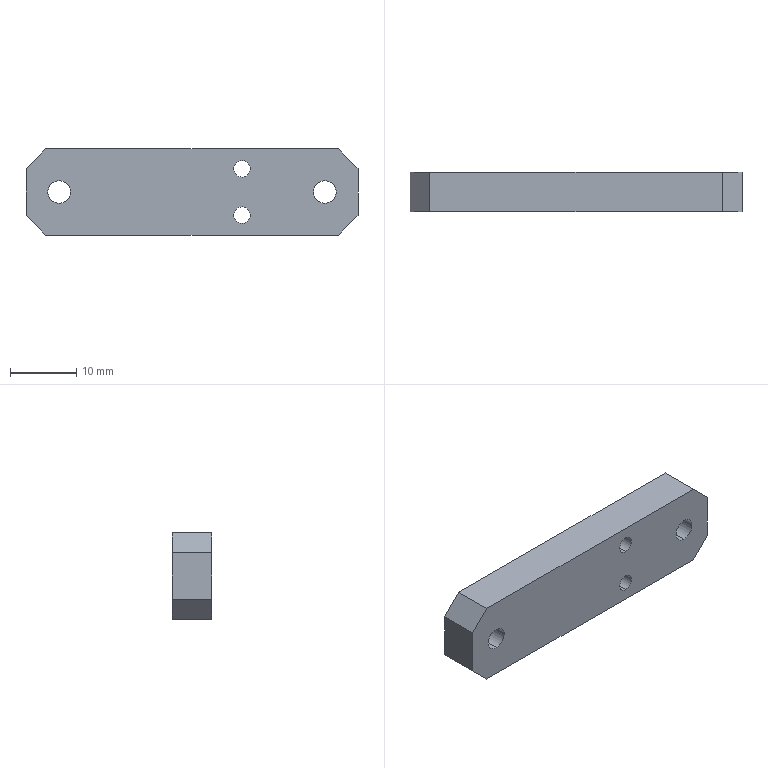Part | NX | features BREP 1 | 1 solid | 24 faces | box 50 x 6 x 13 mm | volume 3494 mm3 | cylinder 12 | plane 12 | commonest cylinder face diameters 2.5 x4 3.4 x4 6 x4
STEP:
#1=CARTESIAN_POINT('',(7.55,-3.,2.252));
#2=VERTEX_POINT('',#1);
#3=CARTESIAN_POINT('',(7.55,-3.,4.752));
#4=VERTEX_POINT('',#3);
#5=CARTESIAN_POINT('',(7.55,-3.,3.502));
#6=DIRECTION('',(0.,1.,0.));
#7=DIRECTION('',(0.,0.,1.));
#8=AXIS2_PLACEMENT_3D('',#5,#6,#7);
#9=CIRCLE('',#8,1.25);
#10=EDGE_CURVE('',#2,#4,#9,.T.);
#11=ORIENTED_EDGE('',*,*,#10,.F.);
#12=CARTESIAN_POINT('',(7.55,3.,2.252));
#13=VERTEX_POINT('',#12);
#14=CARTESIAN_POINT('',(7.55,3.,2.252));
#15=DIRECTION('',(0.,1.,0.));
#16=VECTOR('',#15,1000.);
#17=LINE('',#14,#16);
#18=EDGE_CURVE('',#2,#13,#17,.T.);
#19=ORIENTED_EDGE('',*,*,#18,.T.);
#20=CARTESIAN_POINT('',(7.55,3.,4.752));
#21=VERTEX_POINT('',#20);
#22=CARTESIAN_POINT('',(7.55,3.,3.502));
#23=DIRECTION('',(0.,1.,0.));
#24=DIRECTION('',(0.,0.,1.));
#25=AXIS2_PLACEMENT_3D('',#22,#23,#24);
#26=CIRCLE('',#25,1.25);
#27=EDGE_CURVE('',#13,#21,#26,.T.);
#28=ORIENTED_EDGE('',*,*,#27,.T.);
#29=CARTESIAN_POINT('',(7.55,3.,4.752));
#30=DIRECTION('',(0.,1.,0.));
#31=VECTOR('',#30,1000.);
#32=LINE('',#29,#31);
#33=EDGE_CURVE('',#4,#21,#32,.T.);
#34=ORIENTED_EDGE('',*,*,#33,.F.);
#35=EDGE_LOOP('',(#11,#19,#28,#34));
#36=FACE_BOUND('',#35,.T.);
#37=CARTESIAN_POINT('',(7.55,3.,3.502));
#38=DIRECTION('',(0.,1.,0.));
#39=DIRECTION('',(0.,0.,-1.));
#40=AXIS2_PLACEMENT_3D('',#37,#38,#39);
#41=CYLINDRICAL_SURFACE('',#40,1.25);
#42=ADVANCED_FACE('',(#36),#41,.F.);
#43=CARTESIAN_POINT('',(7.55,-3.,-4.752));
#44=VERTEX_POINT('',#43);
#45=CARTESIAN_POINT('',(7.55,-3.,-2.252));
#46=VERTEX_POINT('',#45);
#47=CARTESIAN_POINT('',(7.55,-3.,-3.502));
#48=DIRECTION('',(0.,1.,0.));
#49=DIRECTION('',(0.,0.,1.));
#50=AXIS2_PLACEMENT_3D('',#47,#48,#49);
#51=CIRCLE('',#50,1.25);
#52=EDGE_CURVE('',#44,#46,#51,.T.);
#53=ORIENTED_EDGE('',*,*,#52,.F.);
#54=CARTESIAN_POINT('',(7.55,3.,-4.752));
#55=VERTEX_POINT('',#54);
#56=CARTESIAN_POINT('',(7.55,3.,-4.752));
#57=DIRECTION('',(0.,1.,0.));
#58=VECTOR('',#57,1000.);
#59=LINE('',#56,#58);
#60=EDGE_CURVE('',#44,#55,#59,.T.);
#61=ORIENTED_EDGE('',*,*,#60,.T.);
#62=CARTESIAN_POINT('',(7.55,3.,-2.252));
#63=VERTEX_POINT('',#62);
#64=CARTESIAN_POINT('',(7.55,3.,-3.502));
#65=DIRECTION('',(0.,1.,0.));
#66=DIRECTION('',(0.,0.,1.));
#67=AXIS2_PLACEMENT_3D('',#64,#65,#66);
#68=CIRCLE('',#67,1.25);
#69=EDGE_CURVE('',#55,#63,#68,.T.);
#70=ORIENTED_EDGE('',*,*,#69,.T.);
#71=CARTESIAN_POINT('',(7.55,3.,-2.252));
#72=DIRECTION('',(0.,1.,0.));
#73=VECTOR('',#72,1000.);
#74=LINE('',#71,#73);
#75=EDGE_CURVE('',#46,#63,#74,.T.);
#76=ORIENTED_EDGE('',*,*,#75,.F.);
#77=EDGE_LOOP('',(#53,#61,#70,#76));
#78=FACE_BOUND('',#77,.T.);
#79=CARTESIAN_POINT('',(7.55,3.,-3.502));
#80=DIRECTION('',(0.,1.,0.));
#81=DIRECTION('',(0.,0.,-1.));
#82=AXIS2_PLACEMENT_3D('',#79,#80,#81);
#83=CYLINDRICAL_SURFACE('',#82,1.25);
#84=ADVANCED_FACE('',(#78),#83,.F.);
#85=CARTESIAN_POINT('',(-20.,-0.4,-3.));
#86=VERTEX_POINT('',#85);
#87=CARTESIAN_POINT('',(-20.,-0.4,3.));
#88=VERTEX_POINT('',#87);
#89=CARTESIAN_POINT('',(-20.,-0.4,0.));
#90=DIRECTION('',(0.,1.,0.));
#91=DIRECTION('',(0.,0.,1.));
#92=AXIS2_PLACEMENT_3D('',#89,#90,#91);
#93=CIRCLE('',#92,3.);
#94=EDGE_CURVE('',#86,#88,#93,.T.);
#95=ORIENTED_EDGE('',*,*,#94,.F.);
#96=CARTESIAN_POINT('',(-20.,3.,-3.));
#97=VERTEX_POINT('',#96);
#98=CARTESIAN_POINT('',(-20.,3.,-3.));
#99=DIRECTION('',(0.,1.,0.));
#100=VECTOR('',#99,1000.);
#101=LINE('',#98,#100);
#102=EDGE_CURVE('',#86,#97,#101,.T.);
#103=ORIENTED_EDGE('',*,*,#102,.T.);
#104=CARTESIAN_POINT('',(-20.,3.,3.));
#105=VERTEX_POINT('',#104);
#106=CARTESIAN_POINT('',(-20.,3.,0.));
#107=DIRECTION('',(0.,1.,0.));
#108=DIRECTION('',(0.,0.,1.));
#109=AXIS2_PLACEMENT_3D('',#106,#107,#108);
#110=CIRCLE('',#109,3.);
#111=EDGE_CURVE('',#97,#105,#110,.T.);
#112=ORIENTED_EDGE('',*,*,#111,.T.);
#113=CARTESIAN_POINT('',(-20.,3.,3.));
#114=DIRECTION('',(0.,1.,0.));
#115=VECTOR('',#114,1000.);
#116=LINE('',#113,#115);
#117=EDGE_CURVE('',#88,#105,#116,.T.);
#118=ORIENTED_EDGE('',*,*,#117,.F.);
#119=EDGE_LOOP('',(#95,#103,#112,#118));
#120=FACE_BOUND('',#119,.T.);
#121=CARTESIAN_POINT('',(-20.,3.,0.));
#122=DIRECTION('',(0.,1.,0.));
#123=DIRECTION('',(0.,0.,-1.));
#124=AXIS2_PLACEMENT_3D('',#121,#122,#123);
#125=CYLINDRICAL_SURFACE('',#124,3.);
#126=ADVANCED_FACE('',(#120),#125,.F.);
#127=CARTESIAN_POINT('',(-20.,-3.,-1.7));
#128=VERTEX_POINT('',#127);
#129=CARTESIAN_POINT('',(-20.,-3.,1.7));
#130=VERTEX_POINT('',#129);
#131=CARTESIAN_POINT('',(-20.,-3.,0.));
#132=DIRECTION('',(0.,1.,0.));
#133=DIRECTION('',(0.,0.,1.));
#134=AXIS2_PLACEMENT_3D('',#131,#132,#133);
#135=CIRCLE('',#134,1.7);
#136=EDGE_CURVE('',#128,#130,#135,.T.);
#137=ORIENTED_EDGE('',*,*,#136,.F.);
#138=CARTESIAN_POINT('',(-20.,-0.4,-1.7));
#139=VERTEX_POINT('',#138);
#140=CARTESIAN_POINT('',(-20.,3.,-1.7));
#141=DIRECTION('',(0.,1.,0.));
#142=VECTOR('',#141,1000.);
#143=LINE('',#140,#142);
#144=EDGE_CURVE('',#128,#139,#143,.T.);
#145=ORIENTED_EDGE('',*,*,#144,.T.);
#146=CARTESIAN_POINT('',(-20.,-0.4,1.7));
#147=VERTEX_POINT('',#146);
#148=CARTESIAN_POINT('',(-20.,-0.4,0.));
#149=DIRECTION('',(0.,1.,0.));
#150=DIRECTION('',(0.,0.,1.));
#151=AXIS2_PLACEMENT_3D('',#148,#149,#150);
#152=CIRCLE('',#151,1.7);
#153=EDGE_CURVE('',#139,#147,#152,.T.);
#154=ORIENTED_EDGE('',*,*,#153,.T.);
#155=CARTESIAN_POINT('',(-20.,3.,1.7));
#156=DIRECTION('',(0.,1.,0.));
#157=VECTOR('',#156,1000.);
#158=LINE('',#155,#157);
#159=EDGE_CURVE('',#130,#147,#158,.T.);
#160=ORIENTED_EDGE('',*,*,#159,.F.);
#161=EDGE_LOOP('',(#137,#145,#154,#160));
#162=FACE_BOUND('',#161,.T.);
#163=CARTESIAN_POINT('',(-20.,3.,0.));
#164=DIRECTION('',(0.,1.,0.));
#165=DIRECTION('',(0.,0.,-1.));
#166=AXIS2_PLACEMENT_3D('',#163,#164,#165);
#167=CYLINDRICAL_SURFACE('',#166,1.7);
#168=ADVANCED_FACE('',(#162),#167,.F.);
#169=CARTESIAN_POINT('',(20.,-0.4,-3.));
#170=VERTEX_POINT('',#169);
#171=CARTESIAN_POINT('',(20.,-0.4,3.));
#172=VERTEX_POINT('',#171);
#173=CARTESIAN_POINT('',(20.,-0.4,0.));
#174=DIRECTION('',(0.,1.,0.));
#175=DIRECTION('',(0.,0.,1.));
#176=AXIS2_PLACEMENT_3D('',#173,#174,#175);
#177=CIRCLE('',#176,3.);
#178=EDGE_CURVE('',#170,#172,#177,.T.);
#179=ORIENTED_EDGE('',*,*,#178,.F.);
#180=CARTESIAN_POINT('',(20.,3.,-3.));
#181=VERTEX_POINT('',#180);
#182=CARTESIAN_POINT('',(20.,3.,-3.));
#183=DIRECTION('',(0.,1.,0.));
#184=VECTOR('',#183,1000.);
#185=LINE('',#182,#184);
#186=EDGE_CURVE('',#170,#181,#185,.T.);
#187=ORIENTED_EDGE('',*,*,#186,.T.);
#188=CARTESIAN_POINT('',(20.,3.,3.));
#189=VERTEX_POINT('',#188);
#190=CARTESIAN_POINT('',(20.,3.,0.));
#191=DIRECTION('',(0.,1.,0.));
#192=DIRECTION('',(0.,0.,1.));
#193=AXIS2_PLACEMENT_3D('',#190,#191,#192);
#194=CIRCLE('',#193,3.);
#195=EDGE_CURVE('',#181,#189,#194,.T.);
#196=ORIENTED_EDGE('',*,*,#195,.T.);
#197=CARTESIAN_POINT('',(20.,3.,3.));
#198=DIRECTION('',(0.,1.,0.));
#199=VECTOR('',#198,1000.);
#200=LINE('',#197,#199);
#201=EDGE_CURVE('',#172,#189,#200,.T.);
#202=ORIENTED_EDGE('',*,*,#201,.F.);
#203=EDGE_LOOP('',(#179,#187,#196,#202));
#204=FACE_BOUND('',#203,.T.);
#205=CARTESIAN_POINT('',(20.,3.,0.));
#206=DIRECTION('',(0.,1.,0.));
#207=DIRECTION('',(0.,0.,-1.));
#208=AXIS2_PLACEMENT_3D('',#205,#206,#207);
#209=CYLINDRICAL_SURFACE('',#208,3.);
#210=ADVANCED_FACE('',(#204),#209,.F.);
#211=CARTESIAN_POINT('',(20.,-3.,-1.7));
#212=VERTEX_POINT('',#211);
#213=CARTESIAN_POINT('',(20.,-3.,1.7));
#214=VERTEX_POINT('',#213);
#215=CARTESIAN_POINT('',(20.,-3.,0.));
#216=DIRECTION('',(0.,1.,0.));
#217=DIRECTION('',(0.,0.,1.));
#218=AXIS2_PLACEMENT_3D('',#215,#216,#217);
#219=CIRCLE('',#218,1.7);
#220=EDGE_CURVE('',#212,#214,#219,.T.);
#221=ORIENTED_EDGE('',*,*,#220,.F.);
#222=CARTESIAN_POINT('',(20.,-0.4,-1.7));
#223=VERTEX_POINT('',#222);
#224=CARTESIAN_POINT('',(20.,3.,-1.7));
#225=DIRECTION('',(0.,1.,0.));
#226=VECTOR('',#225,1000.);
#227=LINE('',#224,#226);
#228=EDGE_CURVE('',#212,#223,#227,.T.);
#229=ORIENTED_EDGE('',*,*,#228,.T.);
#230=CARTESIAN_POINT('',(20.,-0.4,1.7));
#231=VERTEX_POINT('',#230);
#232=CARTESIAN_POINT('',(20.,-0.4,0.));
#233=DIRECTION('',(0.,1.,0.));
#234=DIRECTION('',(0.,0.,1.));
#235=AXIS2_PLACEMENT_3D('',#232,#233,#234);
#236=CIRCLE('',#235,1.7);
#237=EDGE_CURVE('',#223,#231,#236,.T.);
#238=ORIENTED_EDGE('',*,*,#237,.T.);
#239=CARTESIAN_POINT('',(20.,3.,1.7));
#240=DIRECTION('',(0.,1.,0.));
#241=VECTOR('',#240,1000.);
#242=LINE('',#239,#241);
#243=EDGE_CURVE('',#214,#231,#242,.T.);
#244=ORIENTED_EDGE('',*,*,#243,.F.);
#245=EDGE_LOOP('',(#221,#229,#238,#244));
#246=FACE_BOUND('',#245,.T.);
#247=CARTESIAN_POINT('',(20.,3.,0.));
#248=DIRECTION('',(0.,1.,0.));
#249=DIRECTION('',(0.,0.,-1.));
#250=AXIS2_PLACEMENT_3D('',#247,#248,#249);
#251=CYLINDRICAL_SURFACE('',#250,1.7);
#252=ADVANCED_FACE('',(#246),#251,.F.);
#253=CARTESIAN_POINT('',(25.,-3.,3.5));
#254=VERTEX_POINT('',#253);
#255=CARTESIAN_POINT('',(25.,-3.,-3.5));
#256=VERTEX_POINT('',#255);
#257=CARTESIAN_POINT('',(25.,-3.,-6.5));
#258=DIRECTION('',(0.,0.,-1.));
#259=VECTOR('',#258,1000.);
#260=LINE('',#257,#259);
#261=EDGE_CURVE('',#254,#256,#260,.T.);
#262=ORIENTED_EDGE('',*,*,#261,.T.);
#263=CARTESIAN_POINT('',(25.,3.,-3.5));
#264=VERTEX_POINT('',#263);
#265=CARTESIAN_POINT('',(25.,3.,-3.5));
#266=DIRECTION('',(0.,1.,0.));
#267=VECTOR('',#266,1000.);
#268=LINE('',#265,#267);
#269=EDGE_CURVE('',#256,#264,#268,.T.);
#270=ORIENTED_EDGE('',*,*,#269,.T.);
#271=CARTESIAN_POINT('',(25.,3.,3.5));
#272=VERTEX_POINT('',#271);
#273=CARTESIAN_POINT('',(25.,3.,-6.5));
#274=DIRECTION('',(0.,0.,-1.));
#275=VECTOR('',#274,1000.);
#276=LINE('',#273,#275);
#277=EDGE_CURVE('',#272,#264,#276,.T.);
#278=ORIENTED_EDGE('',*,*,#277,.F.);
#279=CARTESIAN_POINT('',(25.,3.,3.5));
#280=DIRECTION('',(0.,-1.,0.));
#281=VECTOR('',#280,1000.);
#282=LINE('',#279,#281);
#283=EDGE_CURVE('',#272,#254,#282,.T.);
#284=ORIENTED_EDGE('',*,*,#283,.T.);
#285=EDGE_LOOP('',(#262,#270,#278,#284));
#286=FACE_BOUND('',#285,.T.);
#287=CARTESIAN_POINT('',(25.,3.,-6.5));
#288=DIRECTION('',(-1.,0.,0.));
#289=DIRECTION('',(0.,0.,-1.));
#290=AXIS2_PLACEMENT_3D('',#287,#288,#289);
#291=PLANE('',#290);
#292=ADVANCED_FACE('',(#286),#291,.F.);
#293=CARTESIAN_POINT('',(22.,-3.,-6.5));
#294=VERTEX_POINT('',#293);
#295=CARTESIAN_POINT('',(-22.,-3.,-6.5));
#296=VERTEX_POINT('',#295);
#297=CARTESIAN_POINT('',(-25.,-3.,-6.5));
#298=DIRECTION('',(-1.,0.,0.));
#299=VECTOR('',#298,1000.);
#300=LINE('',#297,#299);
#301=EDGE_CURVE('',#294,#296,#300,.T.);
#302=ORIENTED_EDGE('',*,*,#301,.T.);
#303=CARTESIAN_POINT('',(-22.,3.,-6.5));
#304=VERTEX_POINT('',#303);
#305=CARTESIAN_POINT('',(-22.,3.,-6.5));
#306=DIRECTION('',(0.,1.,0.));
#307=VECTOR('',#306,1000.);
#308=LINE('',#305,#307);
#309=EDGE_CURVE('',#296,#304,#308,.T.);
#310=ORIENTED_EDGE('',*,*,#309,.T.);
#311=CARTESIAN_POINT('',(22.,3.,-6.5));
#312=VERTEX_POINT('',#311);
#313=CARTESIAN_POINT('',(-25.,3.,-6.5));
#314=DIRECTION('',(-1.,0.,0.));
#315=VECTOR('',#314,1000.);
#316=LINE('',#313,#315);
#317=EDGE_CURVE('',#312,#304,#316,.T.);
#318=ORIENTED_EDGE('',*,*,#317,.F.);
#319=CARTESIAN_POINT('',(22.,3.,-6.5));
#320=DIRECTION('',(0.,-1.,0.));
#321=VECTOR('',#320,1000.);
#322=LINE('',#319,#321);
#323=EDGE_CURVE('',#312,#294,#322,.T.);
#324=ORIENTED_EDGE('',*,*,#323,.T.);
#325=EDGE_LOOP('',(#302,#310,#318,#324));
#326=FACE_BOUND('',#325,.T.);
#327=CARTESIAN_POINT('',(-25.,3.,-6.5));
#328=DIRECTION('',(0.,0.,1.));
#329=DIRECTION('',(-1.,0.,0.));
#330=AXIS2_PLACEMENT_3D('',#327,#328,#329);
#331=PLANE('',#330);
#332=ADVANCED_FACE('',(#326),#331,.F.);
#333=CARTESIAN_POINT('',(-25.,-3.,-3.5));
#334=VERTEX_POINT('',#333);
#335=CARTESIAN_POINT('',(-25.,-3.,3.5));
#336=VERTEX_POINT('',#335);
#337=CARTESIAN_POINT('',(-25.,-3.,-6.5));
#338=DIRECTION('',(0.,0.,1.));
#339=VECTOR('',#338,1000.);
#340=LINE('',#337,#339);
#341=EDGE_CURVE('',#334,#336,#340,.T.);
#342=ORIENTED_EDGE('',*,*,#341,.T.);
#343=CARTESIAN_POINT('',(-25.,3.,3.5));
#344=VERTEX_POINT('',#343);
#345=CARTESIAN_POINT('',(-25.,3.,3.5));
#346=DIRECTION('',(0.,1.,0.));
#347=VECTOR('',#346,1000.);
#348=LINE('',#345,#347);
#349=EDGE_CURVE('',#336,#344,#348,.T.);
#350=ORIENTED_EDGE('',*,*,#349,.T.);
#351=CARTESIAN_POINT('',(-25.,3.,-3.5));
#352=VERTEX_POINT('',#351);
#353=CARTESIAN_POINT('',(-25.,3.,-6.5));
#354=DIRECTION('',(0.,0.,1.));
#355=VECTOR('',#354,1000.);
#356=LINE('',#353,#355);
#357=EDGE_CURVE('',#352,#344,#356,.T.);
#358=ORIENTED_EDGE('',*,*,#357,.F.);
#359=CARTESIAN_POINT('',(-25.,3.,-3.5));
#360=DIRECTION('',(0.,-1.,0.));
#361=VECTOR('',#360,1000.);
#362=LINE('',#359,#361);
#363=EDGE_CURVE('',#352,#334,#362,.T.);
#364=ORIENTED_EDGE('',*,*,#363,.T.);
#365=EDGE_LOOP('',(#342,#350,#358,#364));
#366=FACE_BOUND('',#365,.T.);
#367=CARTESIAN_POINT('',(-25.,3.,-6.5));
#368=DIRECTION('',(1.,0.,0.));
#369=DIRECTION('',(0.,0.,1.));
#370=AXIS2_PLACEMENT_3D('',#367,#368,#369);
#371=PLANE('',#370);
#372=ADVANCED_FACE('',(#366),#371,.F.);
#373=CARTESIAN_POINT('',(-22.,3.,6.5));
#374=VERTEX_POINT('',#373);
#375=CARTESIAN_POINT('',(22.,3.,6.5));
#376=VERTEX_POINT('',#375);
#377=CARTESIAN_POINT('',(-25.,3.,6.5));
#378=DIRECTION('',(1.,0.,0.));
#379=VECTOR('',#378,1000.);
#380=LINE('',#377,#379);
#381=EDGE_CURVE('',#374,#376,#380,.T.);
#382=ORIENTED_EDGE('',*,*,#381,.F.);
#383=CARTESIAN_POINT('',(-22.,-3.,6.5));
#384=VERTEX_POINT('',#383);
#385=CARTESIAN_POINT('',(-22.,3.,6.5));
#386=DIRECTION('',(0.,-1.,0.));
#387=VECTOR('',#386,1000.);
#388=LINE('',#385,#387);
#389=EDGE_CURVE('',#374,#384,#388,.T.);
#390=ORIENTED_EDGE('',*,*,#389,.T.);
#391=CARTESIAN_POINT('',(22.,-3.,6.5));
#392=VERTEX_POINT('',#391);
#393=CARTESIAN_POINT('',(-25.,-3.,6.5));
#394=DIRECTION('',(1.,0.,0.));
#395=VECTOR('',#394,1000.);
#396=LINE('',#393,#395);
#397=EDGE_CURVE('',#384,#392,#396,.T.);
#398=ORIENTED_EDGE('',*,*,#397,.T.);
#399=CARTESIAN_POINT('',(22.,3.,6.5));
#400=DIRECTION('',(0.,1.,0.));
#401=VECTOR('',#400,1000.);
#402=LINE('',#399,#401);
#403=EDGE_CURVE('',#392,#376,#402,.T.);
#404=ORIENTED_EDGE('',*,*,#403,.T.);
#405=EDGE_LOOP('',(#382,#390,#398,#404));
#406=FACE_BOUND('',#405,.T.);
#407=CARTESIAN_POINT('',(-25.,3.,6.5));
#408=DIRECTION('',(0.,0.,-1.));
#409=DIRECTION('',(1.,0.,0.));
#410=AXIS2_PLACEMENT_3D('',#407,#408,#409);
#411=PLANE('',#410);
#412=ADVANCED_FACE('',(#406),#411,.F.);
#413=CARTESIAN_POINT('',(7.55,3.,3.502));
#414=DIRECTION('',(0.,1.,0.));
#415=DIRECTION('',(0.,0.,1.));
#416=AXIS2_PLACEMENT_3D('',#413,#414,#415);
#417=CIRCLE('',#416,1.25);
#418=EDGE_CURVE('',#21,#13,#417,.T.);
#419=ORIENTED_EDGE('',*,*,#418,.F.);
#420=ORIENTED_EDGE('',*,*,#27,.F.);
#421=EDGE_LOOP('',(#419,#420));
#422=FACE_BOUND('',#421,.T.);
#423=CARTESIAN_POINT('',(7.55,3.,-3.502));
#424=DIRECTION('',(0.,1.,0.));
#425=DIRECTION('',(0.,0.,1.));
#426=AXIS2_PLACEMENT_3D('',#423,#424,#425);
#427=CIRCLE('',#426,1.25);
#428=EDGE_CURVE('',#63,#55,#427,.T.);
#429=ORIENTED_EDGE('',*,*,#428,.F.);
#430=ORIENTED_EDGE('',*,*,#69,.F.);
#431=EDGE_LOOP('',(#429,#430));
#432=FACE_BOUND('',#431,.T.);
#433=CARTESIAN_POINT('',(-20.,3.,0.));
#434=DIRECTION('',(0.,1.,0.));
#435=DIRECTION('',(0.,0.,1.));
#436=AXIS2_PLACEMENT_3D('',#433,#434,#435);
#437=CIRCLE('',#436,3.);
#438=EDGE_CURVE('',#105,#97,#437,.T.);
#439=ORIENTED_EDGE('',*,*,#438,.F.);
#440=ORIENTED_EDGE('',*,*,#111,.F.);
#441=EDGE_LOOP('',(#439,#440));
#442=FACE_BOUND('',#441,.T.);
#443=CARTESIAN_POINT('',(20.,3.,0.));
#444=DIRECTION('',(0.,1.,0.));
#445=DIRECTION('',(0.,0.,1.));
#446=AXIS2_PLACEMENT_3D('',#443,#444,#445);
#447=CIRCLE('',#446,3.);
#448=EDGE_CURVE('',#189,#181,#447,.T.);
#449=ORIENTED_EDGE('',*,*,#448,.F.);
#450=ORIENTED_EDGE('',*,*,#195,.F.);
#451=EDGE_LOOP('',(#449,#450));
#452=FACE_BOUND('',#451,.T.);
#453=ORIENTED_EDGE('',*,*,#357,.T.);
#454=CARTESIAN_POINT('',(-14.25,3.,14.25));
#455=DIRECTION('',(0.7071,0.,0.7071));
#456=VECTOR('',#455,1000.);
#457=LINE('',#454,#456);
#458=EDGE_CURVE('',#344,#374,#457,.T.);
#459=ORIENTED_EDGE('',*,*,#458,.T.);
#460=ORIENTED_EDGE('',*,*,#381,.T.);
#461=CARTESIAN_POINT('',(14.25,3.,14.25));
#462=DIRECTION('',(0.7071,0.,-0.7071));
#463=VECTOR('',#462,1000.);
#464=LINE('',#461,#463);
#465=EDGE_CURVE('',#376,#272,#464,.T.);
#466=ORIENTED_EDGE('',*,*,#465,.T.);
#467=ORIENTED_EDGE('',*,*,#277,.T.);
#468=CARTESIAN_POINT('',(14.25,3.,-14.25));
#469=DIRECTION('',(-0.7071,0.,-0.7071));
#470=VECTOR('',#469,1000.);
#471=LINE('',#468,#470);
#472=EDGE_CURVE('',#264,#312,#471,.T.);
#473=ORIENTED_EDGE('',*,*,#472,.T.);
#474=ORIENTED_EDGE('',*,*,#317,.T.);
#475=CARTESIAN_POINT('',(-14.25,3.,-14.25));
#476=DIRECTION('',(-0.7071,0.,0.7071));
#477=VECTOR('',#476,1000.);
#478=LINE('',#475,#477);
#479=EDGE_CURVE('',#304,#352,#478,.T.);
#480=ORIENTED_EDGE('',*,*,#479,.T.);
#481=EDGE_LOOP('',(#453,#459,#460,#466,#467,#473,#474,#480));
#482=FACE_BOUND('',#481,.T.);
#483=CARTESIAN_POINT('',(0.,3.,0.));
#484=DIRECTION('',(0.,1.,0.));
#485=DIRECTION('',(0.,0.,-1.));
#486=AXIS2_PLACEMENT_3D('',#483,#484,#485);
#487=PLANE('',#486);
#488=ADVANCED_FACE('',(#422,#432,#442,#452,#482),#487,.T.);
#489=CARTESIAN_POINT('',(7.55,-3.,3.502));
#490=DIRECTION('',(0.,1.,0.));
#491=DIRECTION('',(0.,0.,1.));
#492=AXIS2_PLACEMENT_3D('',#489,#490,#491);
#493=CIRCLE('',#492,1.25);
#494=EDGE_CURVE('',#4,#2,#493,.T.);
#495=ORIENTED_EDGE('',*,*,#494,.T.);
#496=ORIENTED_EDGE('',*,*,#10,.T.);
#497=EDGE_LOOP('',(#495,#496));
#498=FACE_BOUND('',#497,.T.);
#499=CARTESIAN_POINT('',(7.55,-3.,-3.502));
#500=DIRECTION('',(0.,1.,0.));
#501=DIRECTION('',(0.,0.,1.));
#502=AXIS2_PLACEMENT_3D('',#499,#500,#501);
#503=CIRCLE('',#502,1.25);
#504=EDGE_CURVE('',#46,#44,#503,.T.);
#505=ORIENTED_EDGE('',*,*,#504,.T.);
#506=ORIENTED_EDGE('',*,*,#52,.T.);
#507=EDGE_LOOP('',(#505,#506));
#508=FACE_BOUND('',#507,.T.);
#509=CARTESIAN_POINT('',(-20.,-3.,0.));
#510=DIRECTION('',(0.,1.,0.));
#511=DIRECTION('',(0.,0.,1.));
#512=AXIS2_PLACEMENT_3D('',#509,#510,#511);
#513=CIRCLE('',#512,1.7);
#514=EDGE_CURVE('',#130,#128,#513,.T.);
#515=ORIENTED_EDGE('',*,*,#514,.T.);
#516=ORIENTED_EDGE('',*,*,#136,.T.);
#517=EDGE_LOOP('',(#515,#516));
#518=FACE_BOUND('',#517,.T.);
#519=CARTESIAN_POINT('',(20.,-3.,0.));
#520=DIRECTION('',(0.,1.,0.));
#521=DIRECTION('',(0.,0.,1.));
#522=AXIS2_PLACEMENT_3D('',#519,#520,#521);
#523=CIRCLE('',#522,1.7);
#524=EDGE_CURVE('',#214,#212,#523,.T.);
#525=ORIENTED_EDGE('',*,*,#524,.T.);
#526=ORIENTED_EDGE('',*,*,#220,.T.);
#527=EDGE_LOOP('',(#525,#526));
#528=FACE_BOUND('',#527,.T.);
#529=ORIENTED_EDGE('',*,*,#397,.F.);
#530=CARTESIAN_POINT('',(-22.,-3.,6.5));
#531=DIRECTION('',(-0.7071,0.,-0.7071));
#532=VECTOR('',#531,1000.);
#533=LINE('',#530,#532);
#534=EDGE_CURVE('',#384,#336,#533,.T.);
#535=ORIENTED_EDGE('',*,*,#534,.T.);
#536=ORIENTED_EDGE('',*,*,#341,.F.);
#537=CARTESIAN_POINT('',(-25.,-3.,-3.5));
#538=DIRECTION('',(0.7071,0.,-0.7071));
#539=VECTOR('',#538,1000.);
#540=LINE('',#537,#539);
#541=EDGE_CURVE('',#334,#296,#540,.T.);
#542=ORIENTED_EDGE('',*,*,#541,.T.);
#543=ORIENTED_EDGE('',*,*,#301,.F.);
#544=CARTESIAN_POINT('',(22.,-3.,-6.5));
#545=DIRECTION('',(0.7071,0.,0.7071));
#546=VECTOR('',#545,1000.);
#547=LINE('',#544,#546);
#548=EDGE_CURVE('',#294,#256,#547,.T.);
#549=ORIENTED_EDGE('',*,*,#548,.T.);
#550=ORIENTED_EDGE('',*,*,#261,.F.);
#551=CARTESIAN_POINT('',(25.,-3.,3.5));
#552=DIRECTION('',(-0.7071,0.,0.7071));
#553=VECTOR('',#552,1000.);
#554=LINE('',#551,#553);
#555=EDGE_CURVE('',#254,#392,#554,.T.);
#556=ORIENTED_EDGE('',*,*,#555,.T.);
#557=EDGE_LOOP('',(#529,#535,#536,#542,#543,#549,#550,#556));
#558=FACE_BOUND('',#557,.T.);
#559=CARTESIAN_POINT('',(0.,-3.,0.));
#560=DIRECTION('',(0.,1.,0.));
#561=DIRECTION('',(0.,0.,-1.));
#562=AXIS2_PLACEMENT_3D('',#559,#560,#561);
#563=PLANE('',#562);
#564=ADVANCED_FACE('',(#498,#508,#518,#528,#558),#563,.F.);
#565=ORIENTED_EDGE('',*,*,#228,.F.);
#566=ORIENTED_EDGE('',*,*,#524,.F.);
#567=ORIENTED_EDGE('',*,*,#243,.T.);
#568=CARTESIAN_POINT('',(20.,-0.4,0.));
#569=DIRECTION('',(0.,1.,0.));
#570=DIRECTION('',(0.,0.,1.));
#571=AXIS2_PLACEMENT_3D('',#568,#569,#570);
#572=CIRCLE('',#571,1.7);
#573=EDGE_CURVE('',#231,#223,#572,.T.);
#574=ORIENTED_EDGE('',*,*,#573,.T.);
#575=EDGE_LOOP('',(#565,#566,#567,#574));
#576=FACE_BOUND('',#575,.T.);
#577=CARTESIAN_POINT('',(20.,3.,0.));
#578=DIRECTION('',(0.,1.,0.));
#579=DIRECTION('',(0.,0.,-1.));
#580=AXIS2_PLACEMENT_3D('',#577,#578,#579);
#581=CYLINDRICAL_SURFACE('',#580,1.7);
#582=ADVANCED_FACE('',(#576),#581,.F.);
#583=ORIENTED_EDGE('',*,*,#573,.F.);
#584=ORIENTED_EDGE('',*,*,#237,.F.);
#585=EDGE_LOOP('',(#583,#584));
#586=FACE_BOUND('',#585,.T.);
#587=CARTESIAN_POINT('',(20.,-0.4,0.));
#588=DIRECTION('',(0.,1.,0.));
#589=DIRECTION('',(0.,0.,1.));
#590=AXIS2_PLACEMENT_3D('',#587,#588,#589);
#591=CIRCLE('',#590,3.);
#592=EDGE_CURVE('',#172,#170,#591,.T.);
#593=ORIENTED_EDGE('',*,*,#592,.T.);
#594=ORIENTED_EDGE('',*,*,#178,.T.);
#595=EDGE_LOOP('',(#593,#594));
#596=FACE_BOUND('',#595,.T.);
#597=CARTESIAN_POINT('',(21.7,-0.4,0.));
#598=DIRECTION('',(0.,-1.,0.));
#599=DIRECTION('',(0.,0.,1.));
#600=AXIS2_PLACEMENT_3D('',#597,#598,#599);
#601=PLANE('',#600);
#602=ADVANCED_FACE('',(#586,#596),#601,.F.);
#603=ORIENTED_EDGE('',*,*,#186,.F.);
#604=ORIENTED_EDGE('',*,*,#592,.F.);
#605=ORIENTED_EDGE('',*,*,#201,.T.);
#606=ORIENTED_EDGE('',*,*,#448,.T.);
#607=EDGE_LOOP('',(#603,#604,#605,#606));
#608=FACE_BOUND('',#607,.T.);
#609=CARTESIAN_POINT('',(20.,3.,0.));
#610=DIRECTION('',(0.,1.,0.));
#611=DIRECTION('',(0.,0.,-1.));
#612=AXIS2_PLACEMENT_3D('',#609,#610,#611);
#613=CYLINDRICAL_SURFACE('',#612,3.);
#614=ADVANCED_FACE('',(#608),#613,.F.);
#615=ORIENTED_EDGE('',*,*,#144,.F.);
#616=ORIENTED_EDGE('',*,*,#514,.F.);
#617=ORIENTED_EDGE('',*,*,#159,.T.);
#618=CARTESIAN_POINT('',(-20.,-0.4,0.));
#619=DIRECTION('',(0.,1.,0.));
#620=DIRECTION('',(0.,0.,1.));
#621=AXIS2_PLACEMENT_3D('',#618,#619,#620);
#622=CIRCLE('',#621,1.7);
#623=EDGE_CURVE('',#147,#139,#622,.T.);
#624=ORIENTED_EDGE('',*,*,#623,.T.);
#625=EDGE_LOOP('',(#615,#616,#617,#624));
#626=FACE_BOUND('',#625,.T.);
#627=CARTESIAN_POINT('',(-20.,3.,0.));
#628=DIRECTION('',(0.,1.,0.));
#629=DIRECTION('',(0.,0.,-1.));
#630=AXIS2_PLACEMENT_3D('',#627,#628,#629);
#631=CYLINDRICAL_SURFACE('',#630,1.7);
#632=ADVANCED_FACE('',(#626),#631,.F.);
#633=ORIENTED_EDGE('',*,*,#623,.F.);
#634=ORIENTED_EDGE('',*,*,#153,.F.);
#635=EDGE_LOOP('',(#633,#634));
#636=FACE_BOUND('',#635,.T.);
#637=CARTESIAN_POINT('',(-20.,-0.4,0.));
#638=DIRECTION('',(0.,1.,0.));
#639=DIRECTION('',(0.,0.,1.));
#640=AXIS2_PLACEMENT_3D('',#637,#638,#639);
#641=CIRCLE('',#640,3.);
#642=EDGE_CURVE('',#88,#86,#641,.T.);
#643=ORIENTED_EDGE('',*,*,#642,.T.);
#644=ORIENTED_EDGE('',*,*,#94,.T.);
#645=EDGE_LOOP('',(#643,#644));
#646=FACE_BOUND('',#645,.T.);
#647=CARTESIAN_POINT('',(-18.3,-0.4,0.));
#648=DIRECTION('',(0.,-1.,0.));
#649=DIRECTION('',(0.,0.,1.));
#650=AXIS2_PLACEMENT_3D('',#647,#648,#649);
#651=PLANE('',#650);
#652=ADVANCED_FACE('',(#636,#646),#651,.F.);
#653=ORIENTED_EDGE('',*,*,#102,.F.);
#654=ORIENTED_EDGE('',*,*,#642,.F.);
#655=ORIENTED_EDGE('',*,*,#117,.T.);
#656=ORIENTED_EDGE('',*,*,#438,.T.);
#657=EDGE_LOOP('',(#653,#654,#655,#656));
#658=FACE_BOUND('',#657,.T.);
#659=CARTESIAN_POINT('',(-20.,3.,0.));
#660=DIRECTION('',(0.,1.,0.));
#661=DIRECTION('',(0.,0.,-1.));
#662=AXIS2_PLACEMENT_3D('',#659,#660,#661);
#663=CYLINDRICAL_SURFACE('',#662,3.);
#664=ADVANCED_FACE('',(#658),#663,.F.);
#665=ORIENTED_EDGE('',*,*,#60,.F.);
#666=ORIENTED_EDGE('',*,*,#504,.F.);
#667=ORIENTED_EDGE('',*,*,#75,.T.);
#668=ORIENTED_EDGE('',*,*,#428,.T.);
#669=EDGE_LOOP('',(#665,#666,#667,#668));
#670=FACE_BOUND('',#669,.T.);
#671=CARTESIAN_POINT('',(7.55,3.,-3.502));
#672=DIRECTION('',(0.,1.,0.));
#673=DIRECTION('',(0.,0.,-1.));
#674=AXIS2_PLACEMENT_3D('',#671,#672,#673);
#675=CYLINDRICAL_SURFACE('',#674,1.25);
#676=ADVANCED_FACE('',(#670),#675,.F.);
#677=ORIENTED_EDGE('',*,*,#18,.F.);
#678=ORIENTED_EDGE('',*,*,#494,.F.);
#679=ORIENTED_EDGE('',*,*,#33,.T.);
#680=ORIENTED_EDGE('',*,*,#418,.T.);
#681=EDGE_LOOP('',(#677,#678,#679,#680));
#682=FACE_BOUND('',#681,.T.);
#683=CARTESIAN_POINT('',(7.55,3.,3.502));
#684=DIRECTION('',(0.,1.,0.));
#685=DIRECTION('',(0.,0.,-1.));
#686=AXIS2_PLACEMENT_3D('',#683,#684,#685);
#687=CYLINDRICAL_SURFACE('',#686,1.25);
#688=ADVANCED_FACE('',(#682),#687,.F.);
#689=ORIENTED_EDGE('',*,*,#458,.F.);
#690=ORIENTED_EDGE('',*,*,#349,.F.);
#691=ORIENTED_EDGE('',*,*,#534,.F.);
#692=ORIENTED_EDGE('',*,*,#389,.F.);
#693=EDGE_LOOP('',(#689,#690,#691,#692));
#694=FACE_BOUND('',#693,.T.);
#695=CARTESIAN_POINT('',(-22.,3.,6.5));
#696=DIRECTION('',(0.7071,0.,-0.7071));
#697=DIRECTION('',(0.,1.,0.));
#698=AXIS2_PLACEMENT_3D('',#695,#696,#697);
#699=PLANE('',#698);
#700=ADVANCED_FACE('',(#694),#699,.F.);
#701=ORIENTED_EDGE('',*,*,#479,.F.);
#702=ORIENTED_EDGE('',*,*,#309,.F.);
#703=ORIENTED_EDGE('',*,*,#541,.F.);
#704=ORIENTED_EDGE('',*,*,#363,.F.);
#705=EDGE_LOOP('',(#701,#702,#703,#704));
#706=FACE_BOUND('',#705,.T.);
#707=CARTESIAN_POINT('',(-25.,3.,-3.5));
#708=DIRECTION('',(0.7071,0.,0.7071));
#709=DIRECTION('',(0.,1.,0.));
#710=AXIS2_PLACEMENT_3D('',#707,#708,#709);
#711=PLANE('',#710);
#712=ADVANCED_FACE('',(#706),#711,.F.);
#713=ORIENTED_EDGE('',*,*,#472,.F.);
#714=ORIENTED_EDGE('',*,*,#269,.F.);
#715=ORIENTED_EDGE('',*,*,#548,.F.);
#716=ORIENTED_EDGE('',*,*,#323,.F.);
#717=EDGE_LOOP('',(#713,#714,#715,#716));
#718=FACE_BOUND('',#717,.T.);
#719=CARTESIAN_POINT('',(22.,3.,-6.5));
#720=DIRECTION('',(-0.7071,0.,0.7071));
#721=DIRECTION('',(0.,1.,0.));
#722=AXIS2_PLACEMENT_3D('',#719,#720,#721);
#723=PLANE('',#722);
#724=ADVANCED_FACE('',(#718),#723,.F.);
#725=ORIENTED_EDGE('',*,*,#465,.F.);
#726=ORIENTED_EDGE('',*,*,#403,.F.);
#727=ORIENTED_EDGE('',*,*,#555,.F.);
#728=ORIENTED_EDGE('',*,*,#283,.F.);
#729=EDGE_LOOP('',(#725,#726,#727,#728));
#730=FACE_BOUND('',#729,.T.);
#731=CARTESIAN_POINT('',(25.,3.,3.5));
#732=DIRECTION('',(-0.7071,0.,-0.7071));
#733=DIRECTION('',(0.,1.,0.));
#734=AXIS2_PLACEMENT_3D('',#731,#732,#733);
#735=PLANE('',#734);
#736=ADVANCED_FACE('',(#730),#735,.F.);
#737=CLOSED_SHELL('',(#42,#84,#126,#168,#210,#252,#292,#332,#372,#412,#488,#564,#582,#602,#614,#632,#652,#664,#676,#688,#700,#712,#724,#736));
#738=MANIFOLD_SOLID_BREP('',#737);
#739=(LENGTH_UNIT()NAMED_UNIT(*)SI_UNIT(.MILLI.,.METRE.));
#740=UNCERTAINTY_MEASURE_WITH_UNIT(LENGTH_MEASURE(0.00001),#739,'','');
#741=(NAMED_UNIT(*)PLANE_ANGLE_UNIT()SI_UNIT($,.RADIAN.));
#742=(NAMED_UNIT(*)SI_UNIT($,.STERADIAN.)SOLID_ANGLE_UNIT());
#743=(GEOMETRIC_REPRESENTATION_CONTEXT(3)GLOBAL_UNCERTAINTY_ASSIGNED_CONTEXT((#740))GLOBAL_UNIT_ASSIGNED_CONTEXT((#739,#741,#742))REPRESENTATION_CONTEXT('',''));
#744=ADVANCED_BREP_SHAPE_REPRESENTATION('',(#738),#743);